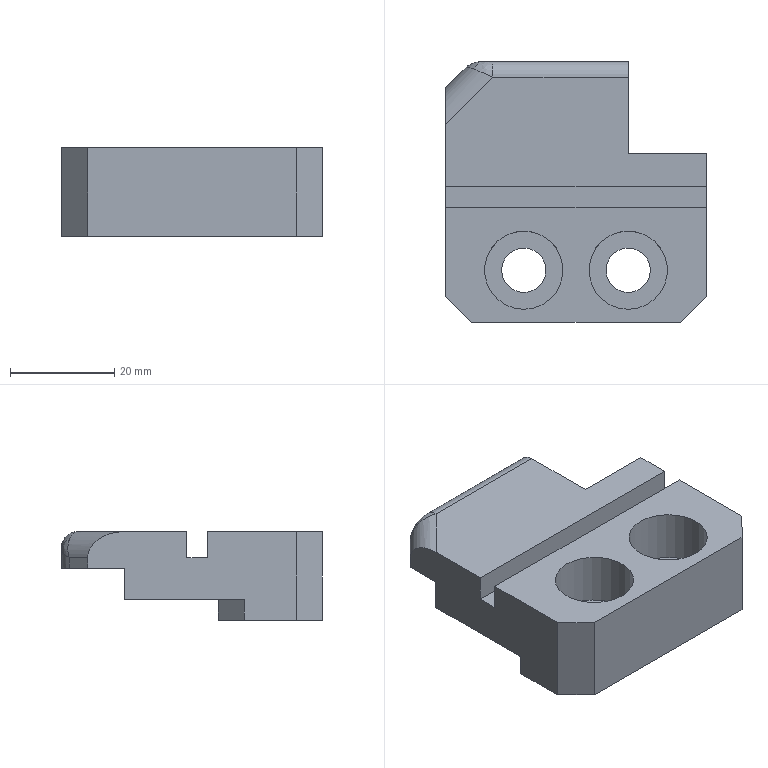Part | STEP file | gslz 2016.10.28-13_id338_x_t | 1 solid | 32 faces | box 50 x 50 x 17 mm | volume 24510 mm3 | plane 23 | cylinder 7 | spline 2 | commonest cylinder face diameters 8.5 x2 10 x2 15 x2 6 x1